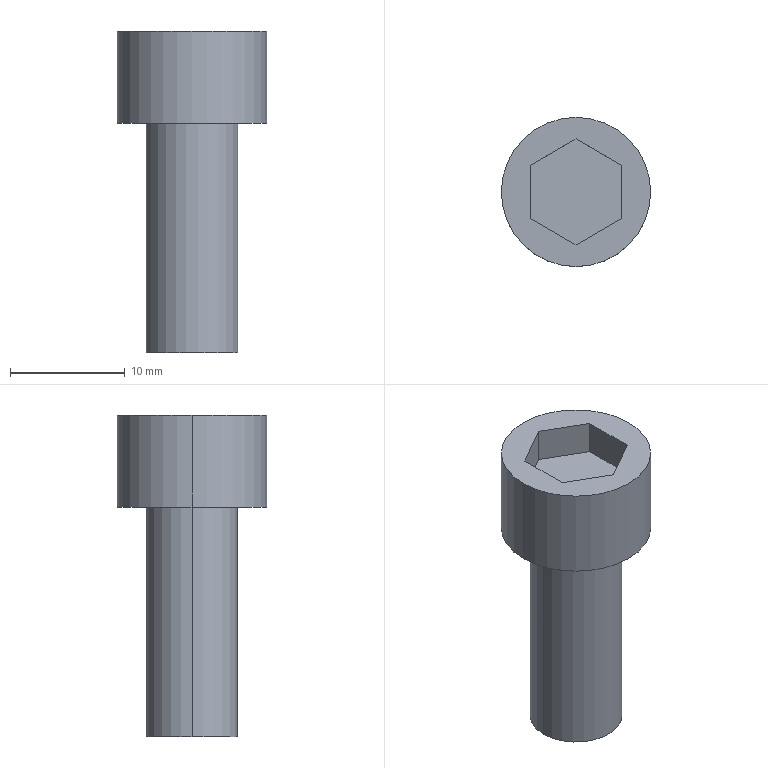Part | STEP file | M8 screw | 1 solid | 14 faces | box 13 x 13 x 28 mm | volume 1901 mm3 | plane 10 | cylinder 4 | commonest cylinder face diameters 8 x2 13 x2
STEP:
#1=CARTESIAN_POINT('',(0.,0.,0.));
#2=DIRECTION('',(0.,0.,1.));
#3=DIRECTION('',(1.,0.,0.));
#4=AXIS2_PLACEMENT_3D('',#1,#2,#3);
#5=CARTESIAN_POINT('',(-4.,0.,-20.));
#6=VERTEX_POINT('',#5);
#7=CARTESIAN_POINT('',(4.,0.,-20.));
#8=VERTEX_POINT('',#7);
#9=CARTESIAN_POINT('',(0.,0.,-20.));
#10=DIRECTION('',(0.,0.,-1.));
#11=DIRECTION('',(-1.,0.,0.));
#12=AXIS2_PLACEMENT_3D('',#9,#10,#11);
#13=CIRCLE('',#12,4.);
#14=CARTESIAN_POINT('',(0.,0.,-20.));
#15=DIRECTION('',(0.,0.,1.));
#16=DIRECTION('',(1.,0.,0.));
#17=AXIS2_PLACEMENT_3D('',#14,#15,#16);
#18=CYLINDRICAL_SURFACE('',#17,4.);
#19=CARTESIAN_POINT('',(3.142,0.));
#20=DIRECTION('',(-1.,0.));
#21=VECTOR('',#20,1.);
#22=LINE('',#19,#21);
#23=(GEOMETRIC_REPRESENTATION_CONTEXT(2)PARAMETRIC_REPRESENTATION_CONTEXT()REPRESENTATION_CONTEXT('',''));
#24=DEFINITIONAL_REPRESENTATION('',(#22),#23);
#25=PCURVE('',#18,#24);
#26=CARTESIAN_POINT('',(0.,0.,-20.));
#27=DIRECTION('',(0.,0.,-1.));
#28=DIRECTION('',(-1.,0.,0.));
#29=AXIS2_PLACEMENT_3D('',#26,#27,#28);
#30=PLANE('',#29);
#31=CARTESIAN_POINT('',(0.,0.));
#32=DIRECTION('',(1.,0.));
#33=AXIS2_PLACEMENT_2D('',#31,#32);
#34=CIRCLE('',#33,4.);
#35=(GEOMETRIC_REPRESENTATION_CONTEXT(2)PARAMETRIC_REPRESENTATION_CONTEXT()REPRESENTATION_CONTEXT('',''));
#36=DEFINITIONAL_REPRESENTATION('',(#34),#35);
#37=PCURVE('',#30,#36);
#38=SURFACE_CURVE('',#13,(#25,#37),.PCURVE_S1.);
#39=EDGE_CURVE('',#6,#8,#38,.T.);
#40=ORIENTED_EDGE('',*,*,#39,.F.);
#41=CARTESIAN_POINT('',(-4.,0.,0.));
#42=VERTEX_POINT('',#41);
#43=CARTESIAN_POINT('',(-4.,0.,-20.));
#44=DIRECTION('',(0.,0.,1.));
#45=VECTOR('',#44,1.);
#46=LINE('',#43,#45);
#47=CARTESIAN_POINT('',(3.142,0.));
#48=DIRECTION('',(0.,1.));
#49=VECTOR('',#48,1.);
#50=LINE('',#47,#49);
#51=(GEOMETRIC_REPRESENTATION_CONTEXT(2)PARAMETRIC_REPRESENTATION_CONTEXT()REPRESENTATION_CONTEXT('',''));
#52=DEFINITIONAL_REPRESENTATION('',(#50),#51);
#53=PCURVE('',#18,#52);
#54=CARTESIAN_POINT('',(0.,0.,-20.));
#55=DIRECTION('',(0.,0.,1.));
#56=DIRECTION('',(1.,0.,0.));
#57=AXIS2_PLACEMENT_3D('',#54,#55,#56);
#58=CYLINDRICAL_SURFACE('',#57,4.);
#59=CARTESIAN_POINT('',(3.142,0.));
#60=DIRECTION('',(0.,1.));
#61=VECTOR('',#60,1.);
#62=LINE('',#59,#61);
#63=(GEOMETRIC_REPRESENTATION_CONTEXT(2)PARAMETRIC_REPRESENTATION_CONTEXT()REPRESENTATION_CONTEXT('',''));
#64=DEFINITIONAL_REPRESENTATION('',(#62),#63);
#65=PCURVE('',#58,#64);
#66=SURFACE_CURVE('',#46,(#53,#65),.PCURVE_S1.);
#67=EDGE_CURVE('',#6,#42,#66,.T.);
#68=ORIENTED_EDGE('',*,*,#67,.T.);
#69=CARTESIAN_POINT('',(4.,0.,0.));
#70=VERTEX_POINT('',#69);
#71=CARTESIAN_POINT('',(0.,0.,0.));
#72=DIRECTION('',(0.,0.,-1.));
#73=DIRECTION('',(1.,0.,0.));
#74=AXIS2_PLACEMENT_3D('',#71,#72,#73);
#75=CIRCLE('',#74,4.);
#76=CARTESIAN_POINT('',(6.283,20.));
#77=DIRECTION('',(-1.,0.));
#78=VECTOR('',#77,1.);
#79=LINE('',#76,#78);
#80=(GEOMETRIC_REPRESENTATION_CONTEXT(2)PARAMETRIC_REPRESENTATION_CONTEXT()REPRESENTATION_CONTEXT('',''));
#81=DEFINITIONAL_REPRESENTATION('',(#79),#80);
#82=PCURVE('',#18,#81);
#83=CARTESIAN_POINT('',(0.,0.,0.));
#84=DIRECTION('',(0.,0.,1.));
#85=DIRECTION('',(1.,0.,0.));
#86=AXIS2_PLACEMENT_3D('',#83,#84,#85);
#87=PLANE('',#86);
#88=CARTESIAN_POINT('',(4.,0.));
#89=CARTESIAN_POINT('',(4.,-6.928));
#90=CARTESIAN_POINT('',(-2.,-3.464));
#91=CARTESIAN_POINT('',(-8.,0.));
#92=CARTESIAN_POINT('',(-2.,3.464));
#93=CARTESIAN_POINT('',(4.,6.928));
#94=CARTESIAN_POINT('',(4.,0.));
#95=(BOUNDED_CURVE()B_SPLINE_CURVE(2,(#88,#89,#90,#91,#92,#93,#94),.UNSPECIFIED.,.T.,.F.)B_SPLINE_CURVE_WITH_KNOTS((1,2,2,2,2,1),(-2.094,0.,2.094,4.189,6.283,8.378),.UNSPECIFIED.)CURVE()GEOMETRIC_REPRESENTATION_ITEM()RATIONAL_B_SPLINE_CURVE((1.,0.5,1.,0.5,1.,0.5,1.))REPRESENTATION_ITEM(''));
#96=(GEOMETRIC_REPRESENTATION_CONTEXT(2)PARAMETRIC_REPRESENTATION_CONTEXT()REPRESENTATION_CONTEXT('',''));
#97=DEFINITIONAL_REPRESENTATION('',(#95),#96);
#98=PCURVE('',#87,#97);
#99=SURFACE_CURVE('',#75,(#82,#98),.PCURVE_S1.);
#100=EDGE_CURVE('',#42,#70,#99,.T.);
#101=ORIENTED_EDGE('',*,*,#100,.T.);
#102=CARTESIAN_POINT('',(4.,0.,-20.));
#103=DIRECTION('',(0.,0.,1.));
#104=VECTOR('',#103,1.);
#105=LINE('',#102,#104);
#106=CARTESIAN_POINT('',(0.,0.));
#107=DIRECTION('',(0.,1.));
#108=VECTOR('',#107,1.);
#109=LINE('',#106,#108);
#110=(GEOMETRIC_REPRESENTATION_CONTEXT(2)PARAMETRIC_REPRESENTATION_CONTEXT()REPRESENTATION_CONTEXT('',''));
#111=DEFINITIONAL_REPRESENTATION('',(#109),#110);
#112=PCURVE('',#18,#111);
#113=CARTESIAN_POINT('',(6.283,0.));
#114=DIRECTION('',(0.,1.));
#115=VECTOR('',#114,1.);
#116=LINE('',#113,#115);
#117=(GEOMETRIC_REPRESENTATION_CONTEXT(2)PARAMETRIC_REPRESENTATION_CONTEXT()REPRESENTATION_CONTEXT('',''));
#118=DEFINITIONAL_REPRESENTATION('',(#116),#117);
#119=PCURVE('',#58,#118);
#120=SURFACE_CURVE('',#105,(#112,#119),.PCURVE_S1.);
#121=EDGE_CURVE('',#8,#70,#120,.T.);
#122=ORIENTED_EDGE('',*,*,#121,.F.);
#123=EDGE_LOOP('',(#40,#68,#101,#122));
#124=FACE_BOUND('',#123,.T.);
#125=ADVANCED_FACE('',(#124),#18,.T.);
#126=CARTESIAN_POINT('',(6.5,0.,8.));
#127=VERTEX_POINT('',#126);
#128=CARTESIAN_POINT('',(-6.5,0.,8.));
#129=VERTEX_POINT('',#128);
#130=CARTESIAN_POINT('',(0.,0.,8.));
#131=DIRECTION('',(0.,0.,1.));
#132=DIRECTION('',(1.,0.,0.));
#133=AXIS2_PLACEMENT_3D('',#130,#131,#132);
#134=CIRCLE('',#133,6.5);
#135=CARTESIAN_POINT('',(0.,0.,8.));
#136=DIRECTION('',(0.,0.,-1.));
#137=DIRECTION('',(-1.,0.,0.));
#138=AXIS2_PLACEMENT_3D('',#135,#136,#137);
#139=CYLINDRICAL_SURFACE('',#138,6.5);
#140=CARTESIAN_POINT('',(3.142,0.));
#141=DIRECTION('',(-1.,0.));
#142=VECTOR('',#141,1.);
#143=LINE('',#140,#142);
#144=(GEOMETRIC_REPRESENTATION_CONTEXT(2)PARAMETRIC_REPRESENTATION_CONTEXT()REPRESENTATION_CONTEXT('',''));
#145=DEFINITIONAL_REPRESENTATION('',(#143),#144);
#146=PCURVE('',#139,#145);
#147=CARTESIAN_POINT('',(0.,0.,8.));
#148=DIRECTION('',(0.,0.,1.));
#149=DIRECTION('',(1.,0.,0.));
#150=AXIS2_PLACEMENT_3D('',#147,#148,#149);
#151=PLANE('',#150);
#152=CARTESIAN_POINT('',(0.,0.));
#153=DIRECTION('',(1.,0.));
#154=AXIS2_PLACEMENT_2D('',#152,#153);
#155=CIRCLE('',#154,6.5);
#156=(GEOMETRIC_REPRESENTATION_CONTEXT(2)PARAMETRIC_REPRESENTATION_CONTEXT()REPRESENTATION_CONTEXT('',''));
#157=DEFINITIONAL_REPRESENTATION('',(#155),#156);
#158=PCURVE('',#151,#157);
#159=SURFACE_CURVE('',#134,(#146,#158),.PCURVE_S1.);
#160=EDGE_CURVE('',#127,#129,#159,.T.);
#161=ORIENTED_EDGE('',*,*,#160,.F.);
#162=CARTESIAN_POINT('',(6.5,0.,0.));
#163=VERTEX_POINT('',#162);
#164=CARTESIAN_POINT('',(6.5,0.,8.));
#165=DIRECTION('',(0.,0.,-1.));
#166=VECTOR('',#165,1.);
#167=LINE('',#164,#166);
#168=CARTESIAN_POINT('',(3.142,0.));
#169=DIRECTION('',(0.,1.));
#170=VECTOR('',#169,1.);
#171=LINE('',#168,#170);
#172=(GEOMETRIC_REPRESENTATION_CONTEXT(2)PARAMETRIC_REPRESENTATION_CONTEXT()REPRESENTATION_CONTEXT('',''));
#173=DEFINITIONAL_REPRESENTATION('',(#171),#172);
#174=PCURVE('',#139,#173);
#175=CARTESIAN_POINT('',(0.,0.,8.));
#176=DIRECTION('',(0.,0.,-1.));
#177=DIRECTION('',(-1.,0.,0.));
#178=AXIS2_PLACEMENT_3D('',#175,#176,#177);
#179=CYLINDRICAL_SURFACE('',#178,6.5);
#180=CARTESIAN_POINT('',(3.142,0.));
#181=DIRECTION('',(0.,1.));
#182=VECTOR('',#181,1.);
#183=LINE('',#180,#182);
#184=(GEOMETRIC_REPRESENTATION_CONTEXT(2)PARAMETRIC_REPRESENTATION_CONTEXT()REPRESENTATION_CONTEXT('',''));
#185=DEFINITIONAL_REPRESENTATION('',(#183),#184);
#186=PCURVE('',#179,#185);
#187=SURFACE_CURVE('',#167,(#174,#186),.PCURVE_S1.);
#188=EDGE_CURVE('',#127,#163,#187,.T.);
#189=ORIENTED_EDGE('',*,*,#188,.T.);
#190=CARTESIAN_POINT('',(-6.5,0.,0.));
#191=VERTEX_POINT('',#190);
#192=CARTESIAN_POINT('',(0.,0.,0.));
#193=DIRECTION('',(0.,0.,1.));
#194=DIRECTION('',(1.,0.,0.));
#195=AXIS2_PLACEMENT_3D('',#192,#193,#194);
#196=CIRCLE('',#195,6.5);
#197=CARTESIAN_POINT('',(3.142,8.));
#198=DIRECTION('',(-1.,0.));
#199=VECTOR('',#198,1.);
#200=LINE('',#197,#199);
#201=(GEOMETRIC_REPRESENTATION_CONTEXT(2)PARAMETRIC_REPRESENTATION_CONTEXT()REPRESENTATION_CONTEXT('',''));
#202=DEFINITIONAL_REPRESENTATION('',(#200),#201);
#203=PCURVE('',#139,#202);
#204=CARTESIAN_POINT('',(0.,0.));
#205=DIRECTION('',(1.,0.));
#206=AXIS2_PLACEMENT_2D('',#204,#205);
#207=CIRCLE('',#206,6.5);
#208=(GEOMETRIC_REPRESENTATION_CONTEXT(2)PARAMETRIC_REPRESENTATION_CONTEXT()REPRESENTATION_CONTEXT('',''));
#209=DEFINITIONAL_REPRESENTATION('',(#207),#208);
#210=PCURVE('',#87,#209);
#211=SURFACE_CURVE('',#196,(#203,#210),.PCURVE_S1.);
#212=EDGE_CURVE('',#163,#191,#211,.T.);
#213=ORIENTED_EDGE('',*,*,#212,.T.);
#214=CARTESIAN_POINT('',(-6.5,0.,8.));
#215=DIRECTION('',(0.,0.,-1.));
#216=VECTOR('',#215,1.);
#217=LINE('',#214,#216);
#218=CARTESIAN_POINT('',(0.,0.));
#219=DIRECTION('',(0.,1.));
#220=VECTOR('',#219,1.);
#221=LINE('',#218,#220);
#222=(GEOMETRIC_REPRESENTATION_CONTEXT(2)PARAMETRIC_REPRESENTATION_CONTEXT()REPRESENTATION_CONTEXT('',''));
#223=DEFINITIONAL_REPRESENTATION('',(#221),#222);
#224=PCURVE('',#139,#223);
#225=CARTESIAN_POINT('',(6.283,0.));
#226=DIRECTION('',(0.,1.));
#227=VECTOR('',#226,1.);
#228=LINE('',#225,#227);
#229=(GEOMETRIC_REPRESENTATION_CONTEXT(2)PARAMETRIC_REPRESENTATION_CONTEXT()REPRESENTATION_CONTEXT('',''));
#230=DEFINITIONAL_REPRESENTATION('',(#228),#229);
#231=PCURVE('',#179,#230);
#232=SURFACE_CURVE('',#217,(#224,#231),.PCURVE_S1.);
#233=EDGE_CURVE('',#129,#191,#232,.T.);
#234=ORIENTED_EDGE('',*,*,#233,.F.);
#235=EDGE_LOOP('',(#161,#189,#213,#234));
#236=FACE_BOUND('',#235,.T.);
#237=ADVANCED_FACE('',(#236),#139,.T.);
#238=CARTESIAN_POINT('',(0.,0.,0.));
#239=DIRECTION('',(0.,0.,1.));
#240=DIRECTION('',(1.,0.,0.));
#241=AXIS2_PLACEMENT_3D('',#238,#239,#240);
#242=CIRCLE('',#241,6.5);
#243=CARTESIAN_POINT('',(0.,0.));
#244=DIRECTION('',(1.,0.));
#245=AXIS2_PLACEMENT_2D('',#243,#244);
#246=CIRCLE('',#245,6.5);
#247=(GEOMETRIC_REPRESENTATION_CONTEXT(2)PARAMETRIC_REPRESENTATION_CONTEXT()REPRESENTATION_CONTEXT('',''));
#248=DEFINITIONAL_REPRESENTATION('',(#246),#247);
#249=PCURVE('',#87,#248);
#250=CARTESIAN_POINT('',(9.425,8.));
#251=DIRECTION('',(-1.,0.));
#252=VECTOR('',#251,1.);
#253=LINE('',#250,#252);
#254=(GEOMETRIC_REPRESENTATION_CONTEXT(2)PARAMETRIC_REPRESENTATION_CONTEXT()REPRESENTATION_CONTEXT('',''));
#255=DEFINITIONAL_REPRESENTATION('',(#253),#254);
#256=PCURVE('',#179,#255);
#257=SURFACE_CURVE('',#242,(#249,#256),.PCURVE_S1.);
#258=EDGE_CURVE('',#191,#163,#257,.T.);
#259=ORIENTED_EDGE('',*,*,#258,.F.);
#260=ORIENTED_EDGE('',*,*,#212,.F.);
#261=EDGE_LOOP('',(#259,#260));
#262=FACE_BOUND('',#261,.T.);
#263=CARTESIAN_POINT('',(0.,0.,0.));
#264=DIRECTION('',(0.,0.,-1.));
#265=DIRECTION('',(1.,0.,0.));
#266=AXIS2_PLACEMENT_3D('',#263,#264,#265);
#267=CIRCLE('',#266,4.);
#268=CARTESIAN_POINT('',(4.,0.));
#269=CARTESIAN_POINT('',(4.,-6.928));
#270=CARTESIAN_POINT('',(-2.,-3.464));
#271=CARTESIAN_POINT('',(-8.,0.));
#272=CARTESIAN_POINT('',(-2.,3.464));
#273=CARTESIAN_POINT('',(4.,6.928));
#274=CARTESIAN_POINT('',(4.,0.));
#275=(BOUNDED_CURVE()B_SPLINE_CURVE(2,(#268,#269,#270,#271,#272,#273,#274),.UNSPECIFIED.,.T.,.F.)B_SPLINE_CURVE_WITH_KNOTS((1,2,2,2,2,1),(-2.094,0.,2.094,4.189,6.283,8.378),.UNSPECIFIED.)CURVE()GEOMETRIC_REPRESENTATION_ITEM()RATIONAL_B_SPLINE_CURVE((1.,0.5,1.,0.5,1.,0.5,1.))REPRESENTATION_ITEM(''));
#276=(GEOMETRIC_REPRESENTATION_CONTEXT(2)PARAMETRIC_REPRESENTATION_CONTEXT()REPRESENTATION_CONTEXT('',''));
#277=DEFINITIONAL_REPRESENTATION('',(#275),#276);
#278=PCURVE('',#87,#277);
#279=CARTESIAN_POINT('',(6.283,20.));
#280=DIRECTION('',(-1.,0.));
#281=VECTOR('',#280,1.);
#282=LINE('',#279,#281);
#283=(GEOMETRIC_REPRESENTATION_CONTEXT(2)PARAMETRIC_REPRESENTATION_CONTEXT()REPRESENTATION_CONTEXT('',''));
#284=DEFINITIONAL_REPRESENTATION('',(#282),#283);
#285=PCURVE('',#58,#284);
#286=SURFACE_CURVE('',#267,(#278,#285),.PCURVE_S1.);
#287=EDGE_CURVE('',#70,#42,#286,.T.);
#288=ORIENTED_EDGE('',*,*,#287,.F.);
#289=ORIENTED_EDGE('',*,*,#100,.F.);
#290=EDGE_LOOP('',(#288,#289));
#291=FACE_BOUND('',#290,.T.);
#292=ADVANCED_FACE('',(#262,#291),#87,.F.);
#293=ORIENTED_EDGE('',*,*,#188,.F.);
#294=CARTESIAN_POINT('',(0.,0.,8.));
#295=DIRECTION('',(0.,0.,1.));
#296=DIRECTION('',(1.,0.,0.));
#297=AXIS2_PLACEMENT_3D('',#294,#295,#296);
#298=CIRCLE('',#297,6.5);
#299=CARTESIAN_POINT('',(9.425,0.));
#300=DIRECTION('',(-1.,0.));
#301=VECTOR('',#300,1.);
#302=LINE('',#299,#301);
#303=(GEOMETRIC_REPRESENTATION_CONTEXT(2)PARAMETRIC_REPRESENTATION_CONTEXT()REPRESENTATION_CONTEXT('',''));
#304=DEFINITIONAL_REPRESENTATION('',(#302),#303);
#305=PCURVE('',#179,#304);
#306=CARTESIAN_POINT('',(0.,0.));
#307=DIRECTION('',(1.,0.));
#308=AXIS2_PLACEMENT_2D('',#306,#307);
#309=CIRCLE('',#308,6.5);
#310=(GEOMETRIC_REPRESENTATION_CONTEXT(2)PARAMETRIC_REPRESENTATION_CONTEXT()REPRESENTATION_CONTEXT('',''));
#311=DEFINITIONAL_REPRESENTATION('',(#309),#310);
#312=PCURVE('',#151,#311);
#313=SURFACE_CURVE('',#298,(#305,#312),.PCURVE_S1.);
#314=EDGE_CURVE('',#129,#127,#313,.T.);
#315=ORIENTED_EDGE('',*,*,#314,.F.);
#316=ORIENTED_EDGE('',*,*,#233,.T.);
#317=ORIENTED_EDGE('',*,*,#258,.T.);
#318=EDGE_LOOP('',(#293,#315,#316,#317));
#319=FACE_BOUND('',#318,.T.);
#320=ADVANCED_FACE('',(#319),#179,.T.);
#321=CARTESIAN_POINT('',(-4.,2.309,8.));
#322=VERTEX_POINT('',#321);
#323=CARTESIAN_POINT('',(-4.,-2.309,8.));
#324=VERTEX_POINT('',#323);
#325=CARTESIAN_POINT('',(-4.,2.309,8.));
#326=DIRECTION('',(0.,-1.,0.));
#327=VECTOR('',#326,1.);
#328=LINE('',#325,#327);
#329=CARTESIAN_POINT('',(-4.,2.309));
#330=DIRECTION('',(0.,-1.));
#331=VECTOR('',#330,1.);
#332=LINE('',#329,#331);
#333=(GEOMETRIC_REPRESENTATION_CONTEXT(2)PARAMETRIC_REPRESENTATION_CONTEXT()REPRESENTATION_CONTEXT('',''));
#334=DEFINITIONAL_REPRESENTATION('',(#332),#333);
#335=PCURVE('',#151,#334);
#336=CARTESIAN_POINT('',(-4.,2.309,5.));
#337=DIRECTION('',(-1.,0.,0.));
#338=DIRECTION('',(0.,0.,1.));
#339=AXIS2_PLACEMENT_3D('',#336,#337,#338);
#340=PLANE('',#339);
#341=CARTESIAN_POINT('',(3.,0.));
#342=DIRECTION('',(0.,-1.));
#343=VECTOR('',#342,1.);
#344=LINE('',#341,#343);
#345=(GEOMETRIC_REPRESENTATION_CONTEXT(2)PARAMETRIC_REPRESENTATION_CONTEXT()REPRESENTATION_CONTEXT('',''));
#346=DEFINITIONAL_REPRESENTATION('',(#344),#345);
#347=PCURVE('',#340,#346);
#348=SURFACE_CURVE('',#328,(#335,#347),.PCURVE_S1.);
#349=EDGE_CURVE('',#322,#324,#348,.T.);
#350=ORIENTED_EDGE('',*,*,#349,.F.);
#351=CARTESIAN_POINT('',(0.,4.619,8.));
#352=VERTEX_POINT('',#351);
#353=CARTESIAN_POINT('',(0.,4.619,8.));
#354=DIRECTION('',(-0.866,-0.5,0.));
#355=VECTOR('',#354,1.);
#356=LINE('',#353,#355);
#357=CARTESIAN_POINT('',(0.,4.619));
#358=DIRECTION('',(-0.866,-0.5));
#359=VECTOR('',#358,1.);
#360=LINE('',#357,#359);
#361=(GEOMETRIC_REPRESENTATION_CONTEXT(2)PARAMETRIC_REPRESENTATION_CONTEXT()REPRESENTATION_CONTEXT('',''));
#362=DEFINITIONAL_REPRESENTATION('',(#360),#361);
#363=PCURVE('',#151,#362);
#364=CARTESIAN_POINT('',(0.,4.619,5.));
#365=DIRECTION('',(-0.5,0.866,0.));
#366=DIRECTION('',(-0.866,-0.5,0.));
#367=AXIS2_PLACEMENT_3D('',#364,#365,#366);
#368=PLANE('',#367);
#369=CARTESIAN_POINT('',(0.,3.));
#370=DIRECTION('',(1.,0.));
#371=VECTOR('',#370,1.);
#372=LINE('',#369,#371);
#373=(GEOMETRIC_REPRESENTATION_CONTEXT(2)PARAMETRIC_REPRESENTATION_CONTEXT()REPRESENTATION_CONTEXT('',''));
#374=DEFINITIONAL_REPRESENTATION('',(#372),#373);
#375=PCURVE('',#368,#374);
#376=SURFACE_CURVE('',#356,(#363,#375),.PCURVE_S1.);
#377=EDGE_CURVE('',#352,#322,#376,.T.);
#378=ORIENTED_EDGE('',*,*,#377,.F.);
#379=CARTESIAN_POINT('',(4.,2.309,8.));
#380=VERTEX_POINT('',#379);
#381=CARTESIAN_POINT('',(4.,2.309,8.));
#382=DIRECTION('',(-0.866,0.5,0.));
#383=VECTOR('',#382,1.);
#384=LINE('',#381,#383);
#385=CARTESIAN_POINT('',(4.,2.309));
#386=DIRECTION('',(-0.866,0.5));
#387=VECTOR('',#386,1.);
#388=LINE('',#385,#387);
#389=(GEOMETRIC_REPRESENTATION_CONTEXT(2)PARAMETRIC_REPRESENTATION_CONTEXT()REPRESENTATION_CONTEXT('',''));
#390=DEFINITIONAL_REPRESENTATION('',(#388),#389);
#391=PCURVE('',#151,#390);
#392=CARTESIAN_POINT('',(4.,2.309,5.));
#393=DIRECTION('',(0.5,0.866,0.));
#394=DIRECTION('',(-0.866,0.5,0.));
#395=AXIS2_PLACEMENT_3D('',#392,#393,#394);
#396=PLANE('',#395);
#397=CARTESIAN_POINT('',(0.,3.));
#398=DIRECTION('',(1.,0.));
#399=VECTOR('',#398,1.);
#400=LINE('',#397,#399);
#401=(GEOMETRIC_REPRESENTATION_CONTEXT(2)PARAMETRIC_REPRESENTATION_CONTEXT()REPRESENTATION_CONTEXT('',''));
#402=DEFINITIONAL_REPRESENTATION('',(#400),#401);
#403=PCURVE('',#396,#402);
#404=SURFACE_CURVE('',#384,(#391,#403),.PCURVE_S1.);
#405=EDGE_CURVE('',#380,#352,#404,.T.);
#406=ORIENTED_EDGE('',*,*,#405,.F.);
#407=CARTESIAN_POINT('',(4.,-2.309,8.));
#408=VERTEX_POINT('',#407);
#409=CARTESIAN_POINT('',(4.,-2.309,8.));
#410=DIRECTION('',(0.,1.,0.));
#411=VECTOR('',#410,1.);
#412=LINE('',#409,#411);
#413=CARTESIAN_POINT('',(4.,-2.309));
#414=DIRECTION('',(0.,1.));
#415=VECTOR('',#414,1.);
#416=LINE('',#413,#415);
#417=(GEOMETRIC_REPRESENTATION_CONTEXT(2)PARAMETRIC_REPRESENTATION_CONTEXT()REPRESENTATION_CONTEXT('',''));
#418=DEFINITIONAL_REPRESENTATION('',(#416),#417);
#419=PCURVE('',#151,#418);
#420=CARTESIAN_POINT('',(4.,-2.309,5.));
#421=DIRECTION('',(1.,0.,0.));
#422=DIRECTION('',(0.,0.,-1.));
#423=AXIS2_PLACEMENT_3D('',#420,#421,#422);
#424=PLANE('',#423);
#425=CARTESIAN_POINT('',(-3.,0.));
#426=DIRECTION('',(0.,1.));
#427=VECTOR('',#426,1.);
#428=LINE('',#425,#427);
#429=(GEOMETRIC_REPRESENTATION_CONTEXT(2)PARAMETRIC_REPRESENTATION_CONTEXT()REPRESENTATION_CONTEXT('',''));
#430=DEFINITIONAL_REPRESENTATION('',(#428),#429);
#431=PCURVE('',#424,#430);
#432=SURFACE_CURVE('',#412,(#419,#431),.PCURVE_S1.);
#433=EDGE_CURVE('',#408,#380,#432,.T.);
#434=ORIENTED_EDGE('',*,*,#433,.F.);
#435=CARTESIAN_POINT('',(0.,-4.619,8.));
#436=VERTEX_POINT('',#435);
#437=CARTESIAN_POINT('',(0.,-4.619,8.));
#438=DIRECTION('',(0.866,0.5,0.));
#439=VECTOR('',#438,1.);
#440=LINE('',#437,#439);
#441=CARTESIAN_POINT('',(0.,-4.619));
#442=DIRECTION('',(0.866,0.5));
#443=VECTOR('',#442,1.);
#444=LINE('',#441,#443);
#445=(GEOMETRIC_REPRESENTATION_CONTEXT(2)PARAMETRIC_REPRESENTATION_CONTEXT()REPRESENTATION_CONTEXT('',''));
#446=DEFINITIONAL_REPRESENTATION('',(#444),#445);
#447=PCURVE('',#151,#446);
#448=CARTESIAN_POINT('',(0.,-4.619,5.));
#449=DIRECTION('',(0.5,-0.866,0.));
#450=DIRECTION('',(0.866,0.5,0.));
#451=AXIS2_PLACEMENT_3D('',#448,#449,#450);
#452=PLANE('',#451);
#453=CARTESIAN_POINT('',(0.,3.));
#454=DIRECTION('',(1.,0.));
#455=VECTOR('',#454,1.);
#456=LINE('',#453,#455);
#457=(GEOMETRIC_REPRESENTATION_CONTEXT(2)PARAMETRIC_REPRESENTATION_CONTEXT()REPRESENTATION_CONTEXT('',''));
#458=DEFINITIONAL_REPRESENTATION('',(#456),#457);
#459=PCURVE('',#452,#458);
#460=SURFACE_CURVE('',#440,(#447,#459),.PCURVE_S1.);
#461=EDGE_CURVE('',#436,#408,#460,.T.);
#462=ORIENTED_EDGE('',*,*,#461,.F.);
#463=CARTESIAN_POINT('',(-4.,-2.309,8.));
#464=DIRECTION('',(0.866,-0.5,0.));
#465=VECTOR('',#464,1.);
#466=LINE('',#463,#465);
#467=CARTESIAN_POINT('',(-4.,-2.309));
#468=DIRECTION('',(0.866,-0.5));
#469=VECTOR('',#468,1.);
#470=LINE('',#467,#469);
#471=(GEOMETRIC_REPRESENTATION_CONTEXT(2)PARAMETRIC_REPRESENTATION_CONTEXT()REPRESENTATION_CONTEXT('',''));
#472=DEFINITIONAL_REPRESENTATION('',(#470),#471);
#473=PCURVE('',#151,#472);
#474=CARTESIAN_POINT('',(-4.,-2.309,5.));
#475=DIRECTION('',(-0.5,-0.866,0.));
#476=DIRECTION('',(0.866,-0.5,0.));
#477=AXIS2_PLACEMENT_3D('',#474,#475,#476);
#478=PLANE('',#477);
#479=CARTESIAN_POINT('',(0.,3.));
#480=DIRECTION('',(1.,0.));
#481=VECTOR('',#480,1.);
#482=LINE('',#479,#481);
#483=(GEOMETRIC_REPRESENTATION_CONTEXT(2)PARAMETRIC_REPRESENTATION_CONTEXT()REPRESENTATION_CONTEXT('',''));
#484=DEFINITIONAL_REPRESENTATION('',(#482),#483);
#485=PCURVE('',#478,#484);
#486=SURFACE_CURVE('',#466,(#473,#485),.PCURVE_S1.);
#487=EDGE_CURVE('',#324,#436,#486,.T.);
#488=ORIENTED_EDGE('',*,*,#487,.F.);
#489=EDGE_LOOP('',(#350,#378,#406,#434,#462,#488));
#490=FACE_BOUND('',#489,.T.);
#491=ORIENTED_EDGE('',*,*,#314,.T.);
#492=ORIENTED_EDGE('',*,*,#160,.T.);
#493=EDGE_LOOP('',(#491,#492));
#494=FACE_BOUND('',#493,.T.);
#495=ADVANCED_FACE('',(#490,#494),#151,.T.);
#496=ORIENTED_EDGE('',*,*,#67,.F.);
#497=CARTESIAN_POINT('',(0.,0.,-20.));
#498=DIRECTION('',(0.,0.,-1.));
#499=DIRECTION('',(-1.,0.,0.));
#500=AXIS2_PLACEMENT_3D('',#497,#498,#499);
#501=CIRCLE('',#500,4.);
#502=CARTESIAN_POINT('',(9.425,0.));
#503=DIRECTION('',(-1.,0.));
#504=VECTOR('',#503,1.);
#505=LINE('',#502,#504);
#506=(GEOMETRIC_REPRESENTATION_CONTEXT(2)PARAMETRIC_REPRESENTATION_CONTEXT()REPRESENTATION_CONTEXT('',''));
#507=DEFINITIONAL_REPRESENTATION('',(#505),#506);
#508=PCURVE('',#58,#507);
#509=CARTESIAN_POINT('',(0.,0.));
#510=DIRECTION('',(1.,0.));
#511=AXIS2_PLACEMENT_2D('',#509,#510);
#512=CIRCLE('',#511,4.);
#513=(GEOMETRIC_REPRESENTATION_CONTEXT(2)PARAMETRIC_REPRESENTATION_CONTEXT()REPRESENTATION_CONTEXT('',''));
#514=DEFINITIONAL_REPRESENTATION('',(#512),#513);
#515=PCURVE('',#30,#514);
#516=SURFACE_CURVE('',#501,(#508,#515),.PCURVE_S1.);
#517=EDGE_CURVE('',#8,#6,#516,.T.);
#518=ORIENTED_EDGE('',*,*,#517,.F.);
#519=ORIENTED_EDGE('',*,*,#121,.T.);
#520=ORIENTED_EDGE('',*,*,#287,.T.);
#521=EDGE_LOOP('',(#496,#518,#519,#520));
#522=FACE_BOUND('',#521,.T.);
#523=ADVANCED_FACE('',(#522),#58,.T.);
#524=ORIENTED_EDGE('',*,*,#517,.T.);
#525=ORIENTED_EDGE('',*,*,#39,.T.);
#526=EDGE_LOOP('',(#524,#525));
#527=FACE_BOUND('',#526,.T.);
#528=ADVANCED_FACE('',(#527),#30,.T.);
#529=ORIENTED_EDGE('',*,*,#349,.T.);
#530=CARTESIAN_POINT('',(-4.,-2.309,5.));
#531=VERTEX_POINT('',#530);
#532=CARTESIAN_POINT('',(-4.,-2.309,5.));
#533=DIRECTION('',(0.,0.,1.));
#534=VECTOR('',#533,1.);
#535=LINE('',#532,#534);
#536=CARTESIAN_POINT('',(0.,-4.619));
#537=DIRECTION('',(1.,0.));
#538=VECTOR('',#537,1.);
#539=LINE('',#536,#538);
#540=(GEOMETRIC_REPRESENTATION_CONTEXT(2)PARAMETRIC_REPRESENTATION_CONTEXT()REPRESENTATION_CONTEXT('',''));
#541=DEFINITIONAL_REPRESENTATION('',(#539),#540);
#542=PCURVE('',#340,#541);
#543=CARTESIAN_POINT('',(0.,0.));
#544=DIRECTION('',(0.,1.));
#545=VECTOR('',#544,1.);
#546=LINE('',#543,#545);
#547=(GEOMETRIC_REPRESENTATION_CONTEXT(2)PARAMETRIC_REPRESENTATION_CONTEXT()REPRESENTATION_CONTEXT('',''));
#548=DEFINITIONAL_REPRESENTATION('',(#546),#547);
#549=PCURVE('',#478,#548);
#550=SURFACE_CURVE('',#535,(#542,#549),.PCURVE_S1.);
#551=EDGE_CURVE('',#531,#324,#550,.T.);
#552=ORIENTED_EDGE('',*,*,#551,.F.);
#553=CARTESIAN_POINT('',(-4.,2.309,5.));
#554=VERTEX_POINT('',#553);
#555=CARTESIAN_POINT('',(-4.,2.309,5.));
#556=DIRECTION('',(0.,-1.,0.));
#557=VECTOR('',#556,1.);
#558=LINE('',#555,#557);
#559=CARTESIAN_POINT('',(0.,0.));
#560=DIRECTION('',(0.,-1.));
#561=VECTOR('',#560,1.);
#562=LINE('',#559,#561);
#563=(GEOMETRIC_REPRESENTATION_CONTEXT(2)PARAMETRIC_REPRESENTATION_CONTEXT()REPRESENTATION_CONTEXT('',''));
#564=DEFINITIONAL_REPRESENTATION('',(#562),#563);
#565=PCURVE('',#340,#564);
#566=CARTESIAN_POINT('',(0.,0.,5.));
#567=DIRECTION('',(0.,0.,1.));
#568=DIRECTION('',(1.,0.,0.));
#569=AXIS2_PLACEMENT_3D('',#566,#567,#568);
#570=PLANE('',#569);
#571=CARTESIAN_POINT('',(-4.,2.309));
#572=DIRECTION('',(0.,-1.));
#573=VECTOR('',#572,1.);
#574=LINE('',#571,#573);
#575=(GEOMETRIC_REPRESENTATION_CONTEXT(2)PARAMETRIC_REPRESENTATION_CONTEXT()REPRESENTATION_CONTEXT('',''));
#576=DEFINITIONAL_REPRESENTATION('',(#574),#575);
#577=PCURVE('',#570,#576);
#578=SURFACE_CURVE('',#558,(#565,#577),.PCURVE_S1.);
#579=EDGE_CURVE('',#554,#531,#578,.T.);
#580=ORIENTED_EDGE('',*,*,#579,.F.);
#581=CARTESIAN_POINT('',(-4.,2.309,5.));
#582=DIRECTION('',(0.,0.,1.));
#583=VECTOR('',#582,1.);
#584=LINE('',#581,#583);
#585=CARTESIAN_POINT('',(0.,0.));
#586=DIRECTION('',(1.,0.));
#587=VECTOR('',#586,1.);
#588=LINE('',#585,#587);
#589=(GEOMETRIC_REPRESENTATION_CONTEXT(2)PARAMETRIC_REPRESENTATION_CONTEXT()REPRESENTATION_CONTEXT('',''));
#590=DEFINITIONAL_REPRESENTATION('',(#588),#589);
#591=PCURVE('',#340,#590);
#592=CARTESIAN_POINT('',(4.619,0.));
#593=DIRECTION('',(0.,1.));
#594=VECTOR('',#593,1.);
#595=LINE('',#592,#594);
#596=(GEOMETRIC_REPRESENTATION_CONTEXT(2)PARAMETRIC_REPRESENTATION_CONTEXT()REPRESENTATION_CONTEXT('',''));
#597=DEFINITIONAL_REPRESENTATION('',(#595),#596);
#598=PCURVE('',#368,#597);
#599=SURFACE_CURVE('',#584,(#591,#598),.PCURVE_S1.);
#600=EDGE_CURVE('',#554,#322,#599,.T.);
#601=ORIENTED_EDGE('',*,*,#600,.T.);
#602=EDGE_LOOP('',(#529,#552,#580,#601));
#603=FACE_BOUND('',#602,.T.);
#604=ADVANCED_FACE('',(#603),#340,.F.);
#605=ORIENTED_EDGE('',*,*,#377,.T.);
#606=ORIENTED_EDGE('',*,*,#600,.F.);
#607=CARTESIAN_POINT('',(0.,4.619,5.));
#608=VERTEX_POINT('',#607);
#609=CARTESIAN_POINT('',(0.,4.619,5.));
#610=DIRECTION('',(-0.866,-0.5,0.));
#611=VECTOR('',#610,1.);
#612=LINE('',#609,#611);
#613=CARTESIAN_POINT('',(0.,0.));
#614=DIRECTION('',(1.,0.));
#615=VECTOR('',#614,1.);
#616=LINE('',#613,#615);
#617=(GEOMETRIC_REPRESENTATION_CONTEXT(2)PARAMETRIC_REPRESENTATION_CONTEXT()REPRESENTATION_CONTEXT('',''));
#618=DEFINITIONAL_REPRESENTATION('',(#616),#617);
#619=PCURVE('',#368,#618);
#620=CARTESIAN_POINT('',(0.,4.619));
#621=DIRECTION('',(-0.866,-0.5));
#622=VECTOR('',#621,1.);
#623=LINE('',#620,#622);
#624=(GEOMETRIC_REPRESENTATION_CONTEXT(2)PARAMETRIC_REPRESENTATION_CONTEXT()REPRESENTATION_CONTEXT('',''));
#625=DEFINITIONAL_REPRESENTATION('',(#623),#624);
#626=PCURVE('',#570,#625);
#627=SURFACE_CURVE('',#612,(#619,#626),.PCURVE_S1.);
#628=EDGE_CURVE('',#608,#554,#627,.T.);
#629=ORIENTED_EDGE('',*,*,#628,.F.);
#630=CARTESIAN_POINT('',(0.,4.619,5.));
#631=DIRECTION('',(0.,0.,1.));
#632=VECTOR('',#631,1.);
#633=LINE('',#630,#632);
#634=CARTESIAN_POINT('',(0.,0.));
#635=DIRECTION('',(0.,1.));
#636=VECTOR('',#635,1.);
#637=LINE('',#634,#636);
#638=(GEOMETRIC_REPRESENTATION_CONTEXT(2)PARAMETRIC_REPRESENTATION_CONTEXT()REPRESENTATION_CONTEXT('',''));
#639=DEFINITIONAL_REPRESENTATION('',(#637),#638);
#640=PCURVE('',#368,#639);
#641=CARTESIAN_POINT('',(4.619,0.));
#642=DIRECTION('',(0.,1.));
#643=VECTOR('',#642,1.);
#644=LINE('',#641,#643);
#645=(GEOMETRIC_REPRESENTATION_CONTEXT(2)PARAMETRIC_REPRESENTATION_CONTEXT()REPRESENTATION_CONTEXT('',''));
#646=DEFINITIONAL_REPRESENTATION('',(#644),#645);
#647=PCURVE('',#396,#646);
#648=SURFACE_CURVE('',#633,(#640,#647),.PCURVE_S1.);
#649=EDGE_CURVE('',#608,#352,#648,.T.);
#650=ORIENTED_EDGE('',*,*,#649,.T.);
#651=EDGE_LOOP('',(#605,#606,#629,#650));
#652=FACE_BOUND('',#651,.T.);
#653=ADVANCED_FACE('',(#652),#368,.F.);
#654=ORIENTED_EDGE('',*,*,#405,.T.);
#655=ORIENTED_EDGE('',*,*,#649,.F.);
#656=CARTESIAN_POINT('',(4.,2.309,5.));
#657=VERTEX_POINT('',#656);
#658=CARTESIAN_POINT('',(4.,2.309,5.));
#659=DIRECTION('',(-0.866,0.5,0.));
#660=VECTOR('',#659,1.);
#661=LINE('',#658,#660);
#662=CARTESIAN_POINT('',(0.,0.));
#663=DIRECTION('',(1.,0.));
#664=VECTOR('',#663,1.);
#665=LINE('',#662,#664);
#666=(GEOMETRIC_REPRESENTATION_CONTEXT(2)PARAMETRIC_REPRESENTATION_CONTEXT()REPRESENTATION_CONTEXT('',''));
#667=DEFINITIONAL_REPRESENTATION('',(#665),#666);
#668=PCURVE('',#396,#667);
#669=CARTESIAN_POINT('',(4.,2.309));
#670=DIRECTION('',(-0.866,0.5));
#671=VECTOR('',#670,1.);
#672=LINE('',#669,#671);
#673=(GEOMETRIC_REPRESENTATION_CONTEXT(2)PARAMETRIC_REPRESENTATION_CONTEXT()REPRESENTATION_CONTEXT('',''));
#674=DEFINITIONAL_REPRESENTATION('',(#672),#673);
#675=PCURVE('',#570,#674);
#676=SURFACE_CURVE('',#661,(#668,#675),.PCURVE_S1.);
#677=EDGE_CURVE('',#657,#608,#676,.T.);
#678=ORIENTED_EDGE('',*,*,#677,.F.);
#679=CARTESIAN_POINT('',(4.,2.309,5.));
#680=DIRECTION('',(0.,0.,1.));
#681=VECTOR('',#680,1.);
#682=LINE('',#679,#681);
#683=CARTESIAN_POINT('',(0.,0.));
#684=DIRECTION('',(0.,1.));
#685=VECTOR('',#684,1.);
#686=LINE('',#683,#685);
#687=(GEOMETRIC_REPRESENTATION_CONTEXT(2)PARAMETRIC_REPRESENTATION_CONTEXT()REPRESENTATION_CONTEXT('',''));
#688=DEFINITIONAL_REPRESENTATION('',(#686),#687);
#689=PCURVE('',#396,#688);
#690=CARTESIAN_POINT('',(0.,4.619));
#691=DIRECTION('',(-1.,0.));
#692=VECTOR('',#691,1.);
#693=LINE('',#690,#692);
#694=(GEOMETRIC_REPRESENTATION_CONTEXT(2)PARAMETRIC_REPRESENTATION_CONTEXT()REPRESENTATION_CONTEXT('',''));
#695=DEFINITIONAL_REPRESENTATION('',(#693),#694);
#696=PCURVE('',#424,#695);
#697=SURFACE_CURVE('',#682,(#689,#696),.PCURVE_S1.);
#698=EDGE_CURVE('',#657,#380,#697,.T.);
#699=ORIENTED_EDGE('',*,*,#698,.T.);
#700=EDGE_LOOP('',(#654,#655,#678,#699));
#701=FACE_BOUND('',#700,.T.);
#702=ADVANCED_FACE('',(#701),#396,.F.);
#703=ORIENTED_EDGE('',*,*,#433,.T.);
#704=ORIENTED_EDGE('',*,*,#698,.F.);
#705=CARTESIAN_POINT('',(4.,-2.309,5.));
#706=VERTEX_POINT('',#705);
#707=CARTESIAN_POINT('',(4.,-2.309,5.));
#708=DIRECTION('',(0.,1.,0.));
#709=VECTOR('',#708,1.);
#710=LINE('',#707,#709);
#711=CARTESIAN_POINT('',(0.,0.));
#712=DIRECTION('',(0.,1.));
#713=VECTOR('',#712,1.);
#714=LINE('',#711,#713);
#715=(GEOMETRIC_REPRESENTATION_CONTEXT(2)PARAMETRIC_REPRESENTATION_CONTEXT()REPRESENTATION_CONTEXT('',''));
#716=DEFINITIONAL_REPRESENTATION('',(#714),#715);
#717=PCURVE('',#424,#716);
#718=CARTESIAN_POINT('',(4.,-2.309));
#719=DIRECTION('',(0.,1.));
#720=VECTOR('',#719,1.);
#721=LINE('',#718,#720);
#722=(GEOMETRIC_REPRESENTATION_CONTEXT(2)PARAMETRIC_REPRESENTATION_CONTEXT()REPRESENTATION_CONTEXT('',''));
#723=DEFINITIONAL_REPRESENTATION('',(#721),#722);
#724=PCURVE('',#570,#723);
#725=SURFACE_CURVE('',#710,(#717,#724),.PCURVE_S1.);
#726=EDGE_CURVE('',#706,#657,#725,.T.);
#727=ORIENTED_EDGE('',*,*,#726,.F.);
#728=CARTESIAN_POINT('',(4.,-2.309,5.));
#729=DIRECTION('',(0.,0.,1.));
#730=VECTOR('',#729,1.);
#731=LINE('',#728,#730);
#732=CARTESIAN_POINT('',(0.,0.));
#733=DIRECTION('',(-1.,0.));
#734=VECTOR('',#733,1.);
#735=LINE('',#732,#734);
#736=(GEOMETRIC_REPRESENTATION_CONTEXT(2)PARAMETRIC_REPRESENTATION_CONTEXT()REPRESENTATION_CONTEXT('',''));
#737=DEFINITIONAL_REPRESENTATION('',(#735),#736);
#738=PCURVE('',#424,#737);
#739=CARTESIAN_POINT('',(4.619,0.));
#740=DIRECTION('',(0.,1.));
#741=VECTOR('',#740,1.);
#742=LINE('',#739,#741);
#743=(GEOMETRIC_REPRESENTATION_CONTEXT(2)PARAMETRIC_REPRESENTATION_CONTEXT()REPRESENTATION_CONTEXT('',''));
#744=DEFINITIONAL_REPRESENTATION('',(#742),#743);
#745=PCURVE('',#452,#744);
#746=SURFACE_CURVE('',#731,(#738,#745),.PCURVE_S1.);
#747=EDGE_CURVE('',#706,#408,#746,.T.);
#748=ORIENTED_EDGE('',*,*,#747,.T.);
#749=EDGE_LOOP('',(#703,#704,#727,#748));
#750=FACE_BOUND('',#749,.T.);
#751=ADVANCED_FACE('',(#750),#424,.F.);
#752=ORIENTED_EDGE('',*,*,#461,.T.);
#753=ORIENTED_EDGE('',*,*,#747,.F.);
#754=CARTESIAN_POINT('',(0.,-4.619,5.));
#755=VERTEX_POINT('',#754);
#756=CARTESIAN_POINT('',(0.,-4.619,5.));
#757=DIRECTION('',(0.866,0.5,0.));
#758=VECTOR('',#757,1.);
#759=LINE('',#756,#758);
#760=CARTESIAN_POINT('',(0.,0.));
#761=DIRECTION('',(1.,0.));
#762=VECTOR('',#761,1.);
#763=LINE('',#760,#762);
#764=(GEOMETRIC_REPRESENTATION_CONTEXT(2)PARAMETRIC_REPRESENTATION_CONTEXT()REPRESENTATION_CONTEXT('',''));
#765=DEFINITIONAL_REPRESENTATION('',(#763),#764);
#766=PCURVE('',#452,#765);
#767=CARTESIAN_POINT('',(0.,-4.619));
#768=DIRECTION('',(0.866,0.5));
#769=VECTOR('',#768,1.);
#770=LINE('',#767,#769);
#771=(GEOMETRIC_REPRESENTATION_CONTEXT(2)PARAMETRIC_REPRESENTATION_CONTEXT()REPRESENTATION_CONTEXT('',''));
#772=DEFINITIONAL_REPRESENTATION('',(#770),#771);
#773=PCURVE('',#570,#772);
#774=SURFACE_CURVE('',#759,(#766,#773),.PCURVE_S1.);
#775=EDGE_CURVE('',#755,#706,#774,.T.);
#776=ORIENTED_EDGE('',*,*,#775,.F.);
#777=CARTESIAN_POINT('',(0.,-4.619,5.));
#778=DIRECTION('',(0.,0.,1.));
#779=VECTOR('',#778,1.);
#780=LINE('',#777,#779);
#781=CARTESIAN_POINT('',(0.,0.));
#782=DIRECTION('',(0.,1.));
#783=VECTOR('',#782,1.);
#784=LINE('',#781,#783);
#785=(GEOMETRIC_REPRESENTATION_CONTEXT(2)PARAMETRIC_REPRESENTATION_CONTEXT()REPRESENTATION_CONTEXT('',''));
#786=DEFINITIONAL_REPRESENTATION('',(#784),#785);
#787=PCURVE('',#452,#786);
#788=CARTESIAN_POINT('',(4.619,0.));
#789=DIRECTION('',(0.,1.));
#790=VECTOR('',#789,1.);
#791=LINE('',#788,#790);
#792=(GEOMETRIC_REPRESENTATION_CONTEXT(2)PARAMETRIC_REPRESENTATION_CONTEXT()REPRESENTATION_CONTEXT('',''));
#793=DEFINITIONAL_REPRESENTATION('',(#791),#792);
#794=PCURVE('',#478,#793);
#795=SURFACE_CURVE('',#780,(#787,#794),.PCURVE_S1.);
#796=EDGE_CURVE('',#755,#436,#795,.T.);
#797=ORIENTED_EDGE('',*,*,#796,.T.);
#798=EDGE_LOOP('',(#752,#753,#776,#797));
#799=FACE_BOUND('',#798,.T.);
#800=ADVANCED_FACE('',(#799),#452,.F.);
#801=ORIENTED_EDGE('',*,*,#487,.T.);
#802=ORIENTED_EDGE('',*,*,#796,.F.);
#803=CARTESIAN_POINT('',(-4.,-2.309,5.));
#804=DIRECTION('',(0.866,-0.5,0.));
#805=VECTOR('',#804,1.);
#806=LINE('',#803,#805);
#807=CARTESIAN_POINT('',(0.,0.));
#808=DIRECTION('',(1.,0.));
#809=VECTOR('',#808,1.);
#810=LINE('',#807,#809);
#811=(GEOMETRIC_REPRESENTATION_CONTEXT(2)PARAMETRIC_REPRESENTATION_CONTEXT()REPRESENTATION_CONTEXT('',''));
#812=DEFINITIONAL_REPRESENTATION('',(#810),#811);
#813=PCURVE('',#478,#812);
#814=CARTESIAN_POINT('',(-4.,-2.309));
#815=DIRECTION('',(0.866,-0.5));
#816=VECTOR('',#815,1.);
#817=LINE('',#814,#816);
#818=(GEOMETRIC_REPRESENTATION_CONTEXT(2)PARAMETRIC_REPRESENTATION_CONTEXT()REPRESENTATION_CONTEXT('',''));
#819=DEFINITIONAL_REPRESENTATION('',(#817),#818);
#820=PCURVE('',#570,#819);
#821=SURFACE_CURVE('',#806,(#813,#820),.PCURVE_S1.);
#822=EDGE_CURVE('',#531,#755,#821,.T.);
#823=ORIENTED_EDGE('',*,*,#822,.F.);
#824=ORIENTED_EDGE('',*,*,#551,.T.);
#825=EDGE_LOOP('',(#801,#802,#823,#824));
#826=FACE_BOUND('',#825,.T.);
#827=ADVANCED_FACE('',(#826),#478,.F.);
#828=ORIENTED_EDGE('',*,*,#579,.T.);
#829=ORIENTED_EDGE('',*,*,#822,.T.);
#830=ORIENTED_EDGE('',*,*,#775,.T.);
#831=ORIENTED_EDGE('',*,*,#726,.T.);
#832=ORIENTED_EDGE('',*,*,#677,.T.);
#833=ORIENTED_EDGE('',*,*,#628,.T.);
#834=EDGE_LOOP('',(#828,#829,#830,#831,#832,#833));
#835=FACE_BOUND('',#834,.T.);
#836=ADVANCED_FACE('',(#835),#570,.T.);
#837=CLOSED_SHELL('',(#125,#237,#292,#320,#495,#523,#528,#604,#653,#702,#751,#800,#827,#836));
#838=MANIFOLD_SOLID_BREP('',#837);
#839=(LENGTH_UNIT()NAMED_UNIT(*)SI_UNIT(.MILLI.,.METRE.));
#840=UNCERTAINTY_MEASURE_WITH_UNIT(LENGTH_MEASURE(0.0000001),#839,'','');
#841=(NAMED_UNIT(*)PLANE_ANGLE_UNIT()SI_UNIT($,.RADIAN.));
#842=(NAMED_UNIT(*)SI_UNIT($,.STERADIAN.)SOLID_ANGLE_UNIT());
#843=(GEOMETRIC_REPRESENTATION_CONTEXT(3)GLOBAL_UNCERTAINTY_ASSIGNED_CONTEXT((#840))GLOBAL_UNIT_ASSIGNED_CONTEXT((#839,#841,#842))REPRESENTATION_CONTEXT('',''));
#844=ADVANCED_BREP_SHAPE_REPRESENTATION('',(#4,#838),#843);